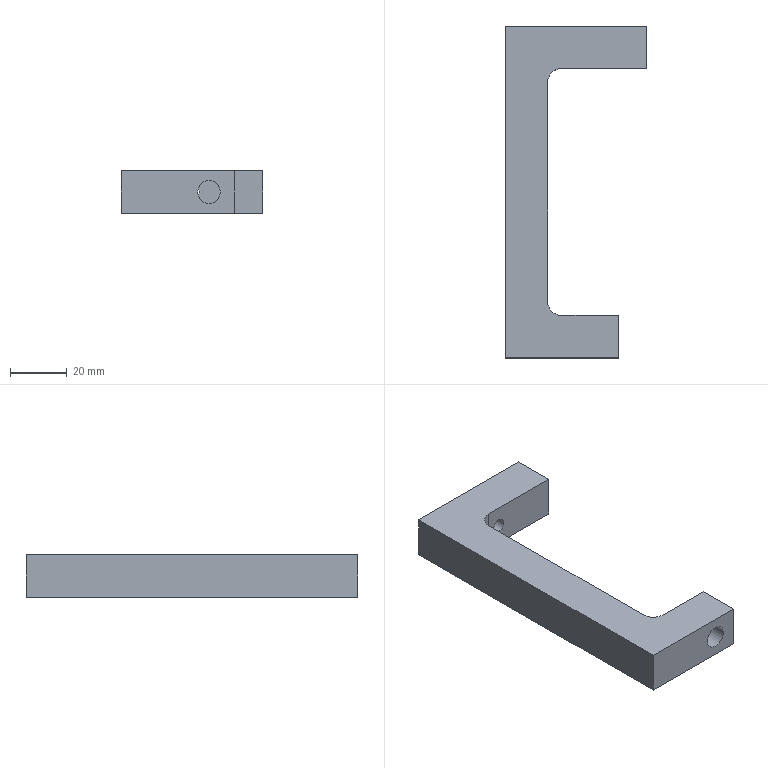Part | NX | features BREP 1 | 1 solid | 18 faces | box 50 x 117 x 15 mm | volume 38225 mm3 | plane 10 | cylinder 6 | cone 2 | commonest cylinder face diameters 6 x2 10 x2 5 x1 8 x1
STEP:
#1=CARTESIAN_POINT('',(50.,102.,0.));
#2=VERTEX_POINT('',#1);
#3=CARTESIAN_POINT('',(50.,117.,0.));
#4=VERTEX_POINT('',#3);
#5=CARTESIAN_POINT('',(50.,102.,0.));
#6=DIRECTION('',(0.,1.,0.));
#7=VECTOR('',#6,1000.);
#8=LINE('',#5,#7);
#9=EDGE_CURVE('',#2,#4,#8,.T.);
#10=ORIENTED_EDGE('',*,*,#9,.T.);
#11=CARTESIAN_POINT('',(50.,117.,15.));
#12=VERTEX_POINT('',#11);
#13=CARTESIAN_POINT('',(50.,117.,15.));
#14=DIRECTION('',(0.,0.,-1.));
#15=VECTOR('',#14,1000.);
#16=LINE('',#13,#15);
#17=EDGE_CURVE('',#12,#4,#16,.T.);
#18=ORIENTED_EDGE('',*,*,#17,.F.);
#19=CARTESIAN_POINT('',(50.,102.,15.));
#20=VERTEX_POINT('',#19);
#21=CARTESIAN_POINT('',(50.,102.,15.));
#22=DIRECTION('',(0.,1.,0.));
#23=VECTOR('',#22,1000.);
#24=LINE('',#21,#23);
#25=EDGE_CURVE('',#20,#12,#24,.T.);
#26=ORIENTED_EDGE('',*,*,#25,.F.);
#27=CARTESIAN_POINT('',(50.,102.,15.));
#28=DIRECTION('',(0.,0.,-1.));
#29=VECTOR('',#28,1000.);
#30=LINE('',#27,#29);
#31=EDGE_CURVE('',#20,#2,#30,.T.);
#32=ORIENTED_EDGE('',*,*,#31,.T.);
#33=EDGE_LOOP('',(#10,#18,#26,#32));
#34=FACE_BOUND('',#33,.T.);
#35=CARTESIAN_POINT('',(50.,102.,15.));
#36=DIRECTION('',(-1.,0.,0.));
#37=DIRECTION('',(0.,1.,0.));
#38=AXIS2_PLACEMENT_3D('',#35,#36,#37);
#39=PLANE('',#38);
#40=ADVANCED_FACE('',(#34),#39,.F.);
#41=CARTESIAN_POINT('',(25.,117.,10.));
#42=VERTEX_POINT('',#41);
#43=CARTESIAN_POINT('',(25.,117.,7.5));
#44=DIRECTION('',(0.,1.,0.));
#45=DIRECTION('',(0.,0.,1.));
#46=AXIS2_PLACEMENT_3D('',#43,#44,#45);
#47=CIRCLE('',#46,2.5);
#48=EDGE_CURVE('',#42,#42,#47,.T.);
#49=ORIENTED_EDGE('',*,*,#48,.F.);
#50=EDGE_LOOP('',(#49));
#51=FACE_BOUND('',#50,.T.);
#52=CARTESIAN_POINT('',(43.,117.,10.5));
#53=VERTEX_POINT('',#52);
#54=CARTESIAN_POINT('',(43.,117.,7.5));
#55=DIRECTION('',(0.,1.,0.));
#56=DIRECTION('',(0.,0.,1.));
#57=AXIS2_PLACEMENT_3D('',#54,#55,#56);
#58=CIRCLE('',#57,3.);
#59=EDGE_CURVE('',#53,#53,#58,.T.);
#60=ORIENTED_EDGE('',*,*,#59,.F.);
#61=EDGE_LOOP('',(#60));
#62=FACE_BOUND('',#61,.T.);
#63=CARTESIAN_POINT('',(7.,117.,10.5));
#64=VERTEX_POINT('',#63);
#65=CARTESIAN_POINT('',(7.,117.,7.5));
#66=DIRECTION('',(0.,1.,0.));
#67=DIRECTION('',(0.,0.,1.));
#68=AXIS2_PLACEMENT_3D('',#65,#66,#67);
#69=CIRCLE('',#68,3.);
#70=EDGE_CURVE('',#64,#64,#69,.T.);
#71=ORIENTED_EDGE('',*,*,#70,.F.);
#72=EDGE_LOOP('',(#71));
#73=FACE_BOUND('',#72,.T.);
#74=CARTESIAN_POINT('',(0.,117.,0.));
#75=VERTEX_POINT('',#74);
#76=CARTESIAN_POINT('',(50.,117.,0.));
#77=DIRECTION('',(-1.,0.,0.));
#78=VECTOR('',#77,1000.);
#79=LINE('',#76,#78);
#80=EDGE_CURVE('',#4,#75,#79,.T.);
#81=ORIENTED_EDGE('',*,*,#80,.T.);
#82=CARTESIAN_POINT('',(0.,117.,15.));
#83=VERTEX_POINT('',#82);
#84=CARTESIAN_POINT('',(0.,117.,15.));
#85=DIRECTION('',(0.,0.,-1.));
#86=VECTOR('',#85,1000.);
#87=LINE('',#84,#86);
#88=EDGE_CURVE('',#83,#75,#87,.T.);
#89=ORIENTED_EDGE('',*,*,#88,.F.);
#90=CARTESIAN_POINT('',(50.,117.,15.));
#91=DIRECTION('',(-1.,0.,0.));
#92=VECTOR('',#91,1000.);
#93=LINE('',#90,#92);
#94=EDGE_CURVE('',#12,#83,#93,.T.);
#95=ORIENTED_EDGE('',*,*,#94,.F.);
#96=ORIENTED_EDGE('',*,*,#17,.T.);
#97=EDGE_LOOP('',(#81,#89,#95,#96));
#98=FACE_BOUND('',#97,.T.);
#99=CARTESIAN_POINT('',(50.,117.,15.));
#100=DIRECTION('',(0.,-1.,0.));
#101=DIRECTION('',(0.,0.,1.));
#102=AXIS2_PLACEMENT_3D('',#99,#100,#101);
#103=PLANE('',#102);
#104=ADVANCED_FACE('',(#51,#62,#73,#98),#103,.F.);
#105=CARTESIAN_POINT('',(0.,0.,0.));
#106=VERTEX_POINT('',#105);
#107=CARTESIAN_POINT('',(0.,117.,0.));
#108=DIRECTION('',(0.,-1.,0.));
#109=VECTOR('',#108,1000.);
#110=LINE('',#107,#109);
#111=EDGE_CURVE('',#75,#106,#110,.T.);
#112=ORIENTED_EDGE('',*,*,#111,.T.);
#113=CARTESIAN_POINT('',(0.,0.,15.));
#114=VERTEX_POINT('',#113);
#115=CARTESIAN_POINT('',(0.,0.,15.));
#116=DIRECTION('',(0.,0.,-1.));
#117=VECTOR('',#116,1000.);
#118=LINE('',#115,#117);
#119=EDGE_CURVE('',#114,#106,#118,.T.);
#120=ORIENTED_EDGE('',*,*,#119,.F.);
#121=CARTESIAN_POINT('',(0.,117.,15.));
#122=DIRECTION('',(0.,-1.,0.));
#123=VECTOR('',#122,1000.);
#124=LINE('',#121,#123);
#125=EDGE_CURVE('',#83,#114,#124,.T.);
#126=ORIENTED_EDGE('',*,*,#125,.F.);
#127=ORIENTED_EDGE('',*,*,#88,.T.);
#128=EDGE_LOOP('',(#112,#120,#126,#127));
#129=FACE_BOUND('',#128,.T.);
#130=CARTESIAN_POINT('',(0.,117.,15.));
#131=DIRECTION('',(1.,0.,0.));
#132=DIRECTION('',(0.,-1.,0.));
#133=AXIS2_PLACEMENT_3D('',#130,#131,#132);
#134=PLANE('',#133);
#135=ADVANCED_FACE('',(#129),#134,.F.);
#136=CARTESIAN_POINT('',(31.,0.,11.5));
#137=VERTEX_POINT('',#136);
#138=CARTESIAN_POINT('',(31.,0.,7.5));
#139=DIRECTION('',(0.,1.,0.));
#140=DIRECTION('',(0.,0.,1.));
#141=AXIS2_PLACEMENT_3D('',#138,#139,#140);
#142=CIRCLE('',#141,4.);
#143=EDGE_CURVE('',#137,#137,#142,.T.);
#144=ORIENTED_EDGE('',*,*,#143,.T.);
#145=EDGE_LOOP('',(#144));
#146=FACE_BOUND('',#145,.T.);
#147=CARTESIAN_POINT('',(40.,0.,0.));
#148=VERTEX_POINT('',#147);
#149=CARTESIAN_POINT('',(0.,0.,0.));
#150=DIRECTION('',(1.,0.,0.));
#151=VECTOR('',#150,1000.);
#152=LINE('',#149,#151);
#153=EDGE_CURVE('',#106,#148,#152,.T.);
#154=ORIENTED_EDGE('',*,*,#153,.T.);
#155=CARTESIAN_POINT('',(40.,0.,15.));
#156=VERTEX_POINT('',#155);
#157=CARTESIAN_POINT('',(40.,0.,15.));
#158=DIRECTION('',(0.,0.,-1.));
#159=VECTOR('',#158,1000.);
#160=LINE('',#157,#159);
#161=EDGE_CURVE('',#156,#148,#160,.T.);
#162=ORIENTED_EDGE('',*,*,#161,.F.);
#163=CARTESIAN_POINT('',(0.,0.,15.));
#164=DIRECTION('',(1.,0.,0.));
#165=VECTOR('',#164,1000.);
#166=LINE('',#163,#165);
#167=EDGE_CURVE('',#114,#156,#166,.T.);
#168=ORIENTED_EDGE('',*,*,#167,.F.);
#169=ORIENTED_EDGE('',*,*,#119,.T.);
#170=EDGE_LOOP('',(#154,#162,#168,#169));
#171=FACE_BOUND('',#170,.T.);
#172=CARTESIAN_POINT('',(0.,0.,15.));
#173=DIRECTION('',(0.,1.,0.));
#174=DIRECTION('',(0.,0.,-1.));
#175=AXIS2_PLACEMENT_3D('',#172,#173,#174);
#176=PLANE('',#175);
#177=ADVANCED_FACE('',(#146,#171),#176,.F.);
#178=CARTESIAN_POINT('',(40.,15.,0.));
#179=VERTEX_POINT('',#178);
#180=CARTESIAN_POINT('',(40.,0.,0.));
#181=DIRECTION('',(0.,1.,0.));
#182=VECTOR('',#181,1000.);
#183=LINE('',#180,#182);
#184=EDGE_CURVE('',#148,#179,#183,.T.);
#185=ORIENTED_EDGE('',*,*,#184,.T.);
#186=CARTESIAN_POINT('',(40.,15.,15.));
#187=VERTEX_POINT('',#186);
#188=CARTESIAN_POINT('',(40.,15.,15.));
#189=DIRECTION('',(0.,0.,-1.));
#190=VECTOR('',#189,1000.);
#191=LINE('',#188,#190);
#192=EDGE_CURVE('',#187,#179,#191,.T.);
#193=ORIENTED_EDGE('',*,*,#192,.F.);
#194=CARTESIAN_POINT('',(40.,0.,15.));
#195=DIRECTION('',(0.,1.,0.));
#196=VECTOR('',#195,1000.);
#197=LINE('',#194,#196);
#198=EDGE_CURVE('',#156,#187,#197,.T.);
#199=ORIENTED_EDGE('',*,*,#198,.F.);
#200=ORIENTED_EDGE('',*,*,#161,.T.);
#201=EDGE_LOOP('',(#185,#193,#199,#200));
#202=FACE_BOUND('',#201,.T.);
#203=CARTESIAN_POINT('',(40.,0.,15.));
#204=DIRECTION('',(-1.,0.,0.));
#205=DIRECTION('',(0.,0.,-1.));
#206=AXIS2_PLACEMENT_3D('',#203,#204,#205);
#207=PLANE('',#206);
#208=ADVANCED_FACE('',(#202),#207,.F.);
#209=CARTESIAN_POINT('',(31.,15.,11.5));
#210=VERTEX_POINT('',#209);
#211=CARTESIAN_POINT('',(31.,15.,7.5));
#212=DIRECTION('',(0.,1.,0.));
#213=DIRECTION('',(0.,0.,1.));
#214=AXIS2_PLACEMENT_3D('',#211,#212,#213);
#215=CIRCLE('',#214,4.);
#216=EDGE_CURVE('',#210,#210,#215,.T.);
#217=ORIENTED_EDGE('',*,*,#216,.F.);
#218=EDGE_LOOP('',(#217));
#219=FACE_BOUND('',#218,.T.);
#220=CARTESIAN_POINT('',(20.,15.,0.));
#221=VERTEX_POINT('',#220);
#222=CARTESIAN_POINT('',(40.,15.,0.));
#223=DIRECTION('',(-1.,0.,0.));
#224=VECTOR('',#223,1000.);
#225=LINE('',#222,#224);
#226=EDGE_CURVE('',#179,#221,#225,.T.);
#227=ORIENTED_EDGE('',*,*,#226,.T.);
#228=CARTESIAN_POINT('',(20.,15.,15.));
#229=VERTEX_POINT('',#228);
#230=CARTESIAN_POINT('',(20.,15.,15.));
#231=DIRECTION('',(0.,0.,1.));
#232=VECTOR('',#231,1000.);
#233=LINE('',#230,#232);
#234=EDGE_CURVE('',#221,#229,#233,.T.);
#235=ORIENTED_EDGE('',*,*,#234,.T.);
#236=CARTESIAN_POINT('',(40.,15.,15.));
#237=DIRECTION('',(-1.,0.,0.));
#238=VECTOR('',#237,1000.);
#239=LINE('',#236,#238);
#240=EDGE_CURVE('',#187,#229,#239,.T.);
#241=ORIENTED_EDGE('',*,*,#240,.F.);
#242=ORIENTED_EDGE('',*,*,#192,.T.);
#243=EDGE_LOOP('',(#227,#235,#241,#242));
#244=FACE_BOUND('',#243,.T.);
#245=CARTESIAN_POINT('',(40.,15.,15.));
#246=DIRECTION('',(0.,-1.,0.));
#247=DIRECTION('',(-1.,0.,0.));
#248=AXIS2_PLACEMENT_3D('',#245,#246,#247);
#249=PLANE('',#248);
#250=ADVANCED_FACE('',(#219,#244),#249,.F.);
#251=CARTESIAN_POINT('',(15.,20.,15.));
#252=VERTEX_POINT('',#251);
#253=CARTESIAN_POINT('',(15.,97.,15.));
#254=VERTEX_POINT('',#253);
#255=CARTESIAN_POINT('',(15.,15.,15.));
#256=DIRECTION('',(0.,1.,0.));
#257=VECTOR('',#256,1000.);
#258=LINE('',#255,#257);
#259=EDGE_CURVE('',#252,#254,#258,.T.);
#260=ORIENTED_EDGE('',*,*,#259,.F.);
#261=CARTESIAN_POINT('',(15.,20.,0.));
#262=VERTEX_POINT('',#261);
#263=CARTESIAN_POINT('',(15.,20.,0.));
#264=DIRECTION('',(0.,0.,-1.));
#265=VECTOR('',#264,1000.);
#266=LINE('',#263,#265);
#267=EDGE_CURVE('',#252,#262,#266,.T.);
#268=ORIENTED_EDGE('',*,*,#267,.T.);
#269=CARTESIAN_POINT('',(15.,97.,0.));
#270=VERTEX_POINT('',#269);
#271=CARTESIAN_POINT('',(15.,15.,0.));
#272=DIRECTION('',(0.,1.,0.));
#273=VECTOR('',#272,1000.);
#274=LINE('',#271,#273);
#275=EDGE_CURVE('',#262,#270,#274,.T.);
#276=ORIENTED_EDGE('',*,*,#275,.T.);
#277=CARTESIAN_POINT('',(15.,97.,15.));
#278=DIRECTION('',(0.,0.,1.));
#279=VECTOR('',#278,1000.);
#280=LINE('',#277,#279);
#281=EDGE_CURVE('',#270,#254,#280,.T.);
#282=ORIENTED_EDGE('',*,*,#281,.T.);
#283=EDGE_LOOP('',(#260,#268,#276,#282));
#284=FACE_BOUND('',#283,.T.);
#285=CARTESIAN_POINT('',(15.,15.,15.));
#286=DIRECTION('',(-1.,0.,0.));
#287=DIRECTION('',(0.,0.,-1.));
#288=AXIS2_PLACEMENT_3D('',#285,#286,#287);
#289=PLANE('',#288);
#290=ADVANCED_FACE('',(#284),#289,.F.);
#291=CARTESIAN_POINT('',(25.,102.,10.));
#292=VERTEX_POINT('',#291);
#293=CARTESIAN_POINT('',(25.,102.,7.5));
#294=DIRECTION('',(0.,1.,0.));
#295=DIRECTION('',(0.,0.,1.));
#296=AXIS2_PLACEMENT_3D('',#293,#294,#295);
#297=CIRCLE('',#296,2.5);
#298=EDGE_CURVE('',#292,#292,#297,.T.);
#299=ORIENTED_EDGE('',*,*,#298,.T.);
#300=EDGE_LOOP('',(#299));
#301=FACE_BOUND('',#300,.T.);
#302=CARTESIAN_POINT('',(20.,102.,15.));
#303=VERTEX_POINT('',#302);
#304=CARTESIAN_POINT('',(15.,102.,15.));
#305=DIRECTION('',(1.,0.,0.));
#306=VECTOR('',#305,1000.);
#307=LINE('',#304,#306);
#308=EDGE_CURVE('',#303,#20,#307,.T.);
#309=ORIENTED_EDGE('',*,*,#308,.F.);
#310=CARTESIAN_POINT('',(20.,102.,0.));
#311=VERTEX_POINT('',#310);
#312=CARTESIAN_POINT('',(20.,102.,0.));
#313=DIRECTION('',(0.,0.,-1.));
#314=VECTOR('',#313,1000.);
#315=LINE('',#312,#314);
#316=EDGE_CURVE('',#303,#311,#315,.T.);
#317=ORIENTED_EDGE('',*,*,#316,.T.);
#318=CARTESIAN_POINT('',(15.,102.,0.));
#319=DIRECTION('',(1.,0.,0.));
#320=VECTOR('',#319,1000.);
#321=LINE('',#318,#320);
#322=EDGE_CURVE('',#311,#2,#321,.T.);
#323=ORIENTED_EDGE('',*,*,#322,.T.);
#324=ORIENTED_EDGE('',*,*,#31,.F.);
#325=EDGE_LOOP('',(#309,#317,#323,#324));
#326=FACE_BOUND('',#325,.T.);
#327=CARTESIAN_POINT('',(15.,102.,15.));
#328=DIRECTION('',(0.,1.,0.));
#329=DIRECTION('',(0.,0.,-1.));
#330=AXIS2_PLACEMENT_3D('',#327,#328,#329);
#331=PLANE('',#330);
#332=ADVANCED_FACE('',(#301,#326),#331,.F.);
#333=ORIENTED_EDGE('',*,*,#25,.T.);
#334=ORIENTED_EDGE('',*,*,#94,.T.);
#335=ORIENTED_EDGE('',*,*,#125,.T.);
#336=ORIENTED_EDGE('',*,*,#167,.T.);
#337=ORIENTED_EDGE('',*,*,#198,.T.);
#338=ORIENTED_EDGE('',*,*,#240,.T.);
#339=CARTESIAN_POINT('',(20.,20.,15.));
#340=DIRECTION('',(0.,0.,-1.));
#341=DIRECTION('',(1.,0.,0.));
#342=AXIS2_PLACEMENT_3D('',#339,#340,#341);
#343=CIRCLE('',#342,5.);
#344=EDGE_CURVE('',#229,#252,#343,.T.);
#345=ORIENTED_EDGE('',*,*,#344,.T.);
#346=ORIENTED_EDGE('',*,*,#259,.T.);
#347=CARTESIAN_POINT('',(20.,97.,15.));
#348=DIRECTION('',(0.,0.,-1.));
#349=DIRECTION('',(1.,0.,0.));
#350=AXIS2_PLACEMENT_3D('',#347,#348,#349);
#351=CIRCLE('',#350,5.);
#352=EDGE_CURVE('',#254,#303,#351,.T.);
#353=ORIENTED_EDGE('',*,*,#352,.T.);
#354=ORIENTED_EDGE('',*,*,#308,.T.);
#355=EDGE_LOOP('',(#333,#334,#335,#336,#337,#338,#345,#346,#353,#354));
#356=FACE_BOUND('',#355,.T.);
#357=CARTESIAN_POINT('',(0.,0.,15.));
#358=DIRECTION('',(0.,0.,1.));
#359=DIRECTION('',(-1.,0.,0.));
#360=AXIS2_PLACEMENT_3D('',#357,#358,#359);
#361=PLANE('',#360);
#362=ADVANCED_FACE('',(#356),#361,.T.);
#363=ORIENTED_EDGE('',*,*,#9,.F.);
#364=ORIENTED_EDGE('',*,*,#322,.F.);
#365=CARTESIAN_POINT('',(20.,97.,0.));
#366=DIRECTION('',(0.,0.,1.));
#367=DIRECTION('',(1.,0.,0.));
#368=AXIS2_PLACEMENT_3D('',#365,#366,#367);
#369=CIRCLE('',#368,5.);
#370=EDGE_CURVE('',#311,#270,#369,.T.);
#371=ORIENTED_EDGE('',*,*,#370,.T.);
#372=ORIENTED_EDGE('',*,*,#275,.F.);
#373=CARTESIAN_POINT('',(20.,20.,0.));
#374=DIRECTION('',(0.,0.,1.));
#375=DIRECTION('',(1.,0.,0.));
#376=AXIS2_PLACEMENT_3D('',#373,#374,#375);
#377=CIRCLE('',#376,5.);
#378=EDGE_CURVE('',#262,#221,#377,.T.);
#379=ORIENTED_EDGE('',*,*,#378,.T.);
#380=ORIENTED_EDGE('',*,*,#226,.F.);
#381=ORIENTED_EDGE('',*,*,#184,.F.);
#382=ORIENTED_EDGE('',*,*,#153,.F.);
#383=ORIENTED_EDGE('',*,*,#111,.F.);
#384=ORIENTED_EDGE('',*,*,#80,.F.);
#385=EDGE_LOOP('',(#363,#364,#371,#372,#379,#380,#381,#382,#383,#384));
#386=FACE_BOUND('',#385,.T.);
#387=CARTESIAN_POINT('',(0.,0.,0.));
#388=DIRECTION('',(0.,0.,1.));
#389=DIRECTION('',(-1.,0.,0.));
#390=AXIS2_PLACEMENT_3D('',#387,#388,#389);
#391=PLANE('',#390);
#392=ADVANCED_FACE('',(#386),#391,.F.);
#393=ORIENTED_EDGE('',*,*,#344,.F.);
#394=ORIENTED_EDGE('',*,*,#234,.F.);
#395=ORIENTED_EDGE('',*,*,#378,.F.);
#396=ORIENTED_EDGE('',*,*,#267,.F.);
#397=EDGE_LOOP('',(#393,#394,#395,#396));
#398=FACE_BOUND('',#397,.T.);
#399=CARTESIAN_POINT('',(20.,20.,15.));
#400=DIRECTION('',(0.,0.,1.));
#401=DIRECTION('',(-1.,0.,0.));
#402=AXIS2_PLACEMENT_3D('',#399,#400,#401);
#403=CYLINDRICAL_SURFACE('',#402,5.);
#404=ADVANCED_FACE('',(#398),#403,.F.);
#405=ORIENTED_EDGE('',*,*,#352,.F.);
#406=ORIENTED_EDGE('',*,*,#281,.F.);
#407=ORIENTED_EDGE('',*,*,#370,.F.);
#408=ORIENTED_EDGE('',*,*,#316,.F.);
#409=EDGE_LOOP('',(#405,#406,#407,#408));
#410=FACE_BOUND('',#409,.T.);
#411=CARTESIAN_POINT('',(20.,97.,15.));
#412=DIRECTION('',(0.,0.,1.));
#413=DIRECTION('',(-1.,0.,0.));
#414=AXIS2_PLACEMENT_3D('',#411,#412,#413);
#415=CYLINDRICAL_SURFACE('',#414,5.);
#416=ADVANCED_FACE('',(#410),#415,.F.);
#417=CARTESIAN_POINT('',(7.,103.197,7.5));
#418=VERTEX_POINT('',#417);
#419=VERTEX_LOOP('',#418);
#420=FACE_BOUND('',#419,.T.);
#421=CARTESIAN_POINT('',(7.,105.,10.5));
#422=VERTEX_POINT('',#421);
#423=CARTESIAN_POINT('',(7.,105.,7.5));
#424=DIRECTION('',(0.,1.,0.));
#425=DIRECTION('',(0.,0.,1.));
#426=AXIS2_PLACEMENT_3D('',#423,#424,#425);
#427=CIRCLE('',#426,3.);
#428=EDGE_CURVE('',#422,#422,#427,.T.);
#429=ORIENTED_EDGE('',*,*,#428,.T.);
#430=EDGE_LOOP('',(#429));
#431=FACE_BOUND('',#430,.T.);
#432=CARTESIAN_POINT('',(7.,105.,7.5));
#433=DIRECTION('',(0.,1.,0.));
#434=DIRECTION('',(0.,0.,-1.));
#435=AXIS2_PLACEMENT_3D('',#432,#433,#434);
#436=CONICAL_SURFACE('',#435,3.,1.03);
#437=ADVANCED_FACE('',(#420,#431),#436,.F.);
#438=ORIENTED_EDGE('',*,*,#428,.F.);
#439=EDGE_LOOP('',(#438));
#440=FACE_BOUND('',#439,.T.);
#441=ORIENTED_EDGE('',*,*,#70,.T.);
#442=EDGE_LOOP('',(#441));
#443=FACE_BOUND('',#442,.T.);
#444=CARTESIAN_POINT('',(7.,117.,7.5));
#445=DIRECTION('',(0.,1.,0.));
#446=DIRECTION('',(0.,0.,-1.));
#447=AXIS2_PLACEMENT_3D('',#444,#445,#446);
#448=CYLINDRICAL_SURFACE('',#447,3.);
#449=ADVANCED_FACE('',(#440,#443),#448,.F.);
#450=CARTESIAN_POINT('',(43.,103.197,7.5));
#451=VERTEX_POINT('',#450);
#452=VERTEX_LOOP('',#451);
#453=FACE_BOUND('',#452,.T.);
#454=CARTESIAN_POINT('',(43.,105.,10.5));
#455=VERTEX_POINT('',#454);
#456=CARTESIAN_POINT('',(43.,105.,7.5));
#457=DIRECTION('',(0.,1.,0.));
#458=DIRECTION('',(0.,0.,1.));
#459=AXIS2_PLACEMENT_3D('',#456,#457,#458);
#460=CIRCLE('',#459,3.);
#461=EDGE_CURVE('',#455,#455,#460,.T.);
#462=ORIENTED_EDGE('',*,*,#461,.T.);
#463=EDGE_LOOP('',(#462));
#464=FACE_BOUND('',#463,.T.);
#465=CARTESIAN_POINT('',(43.,105.,7.5));
#466=DIRECTION('',(0.,1.,0.));
#467=DIRECTION('',(0.,0.,-1.));
#468=AXIS2_PLACEMENT_3D('',#465,#466,#467);
#469=CONICAL_SURFACE('',#468,3.,1.03);
#470=ADVANCED_FACE('',(#453,#464),#469,.F.);
#471=ORIENTED_EDGE('',*,*,#461,.F.);
#472=EDGE_LOOP('',(#471));
#473=FACE_BOUND('',#472,.T.);
#474=ORIENTED_EDGE('',*,*,#59,.T.);
#475=EDGE_LOOP('',(#474));
#476=FACE_BOUND('',#475,.T.);
#477=CARTESIAN_POINT('',(43.,117.,7.5));
#478=DIRECTION('',(0.,1.,0.));
#479=DIRECTION('',(0.,0.,-1.));
#480=AXIS2_PLACEMENT_3D('',#477,#478,#479);
#481=CYLINDRICAL_SURFACE('',#480,3.);
#482=ADVANCED_FACE('',(#473,#476),#481,.F.);
#483=ORIENTED_EDGE('',*,*,#298,.F.);
#484=EDGE_LOOP('',(#483));
#485=FACE_BOUND('',#484,.T.);
#486=ORIENTED_EDGE('',*,*,#48,.T.);
#487=EDGE_LOOP('',(#486));
#488=FACE_BOUND('',#487,.T.);
#489=CARTESIAN_POINT('',(25.,117.,7.5));
#490=DIRECTION('',(0.,1.,0.));
#491=DIRECTION('',(0.,0.,-1.));
#492=AXIS2_PLACEMENT_3D('',#489,#490,#491);
#493=CYLINDRICAL_SURFACE('',#492,2.5);
#494=ADVANCED_FACE('',(#485,#488),#493,.F.);
#495=ORIENTED_EDGE('',*,*,#143,.F.);
#496=EDGE_LOOP('',(#495));
#497=FACE_BOUND('',#496,.T.);
#498=ORIENTED_EDGE('',*,*,#216,.T.);
#499=EDGE_LOOP('',(#498));
#500=FACE_BOUND('',#499,.T.);
#501=CARTESIAN_POINT('',(31.,15.,7.5));
#502=DIRECTION('',(0.,1.,0.));
#503=DIRECTION('',(0.,0.,-1.));
#504=AXIS2_PLACEMENT_3D('',#501,#502,#503);
#505=CYLINDRICAL_SURFACE('',#504,4.);
#506=ADVANCED_FACE('',(#497,#500),#505,.F.);
#507=CLOSED_SHELL('',(#40,#104,#135,#177,#208,#250,#290,#332,#362,#392,#404,#416,#437,#449,#470,#482,#494,#506));
#508=MANIFOLD_SOLID_BREP('',#507);
#509=(LENGTH_UNIT()NAMED_UNIT(*)SI_UNIT(.MILLI.,.METRE.));
#510=UNCERTAINTY_MEASURE_WITH_UNIT(LENGTH_MEASURE(0.00001),#509,'','');
#511=(NAMED_UNIT(*)PLANE_ANGLE_UNIT()SI_UNIT($,.RADIAN.));
#512=(NAMED_UNIT(*)SI_UNIT($,.STERADIAN.)SOLID_ANGLE_UNIT());
#513=(GEOMETRIC_REPRESENTATION_CONTEXT(3)GLOBAL_UNCERTAINTY_ASSIGNED_CONTEXT((#510))GLOBAL_UNIT_ASSIGNED_CONTEXT((#509,#511,#512))REPRESENTATION_CONTEXT('',''));
#514=ADVANCED_BREP_SHAPE_REPRESENTATION('',(#508),#513);